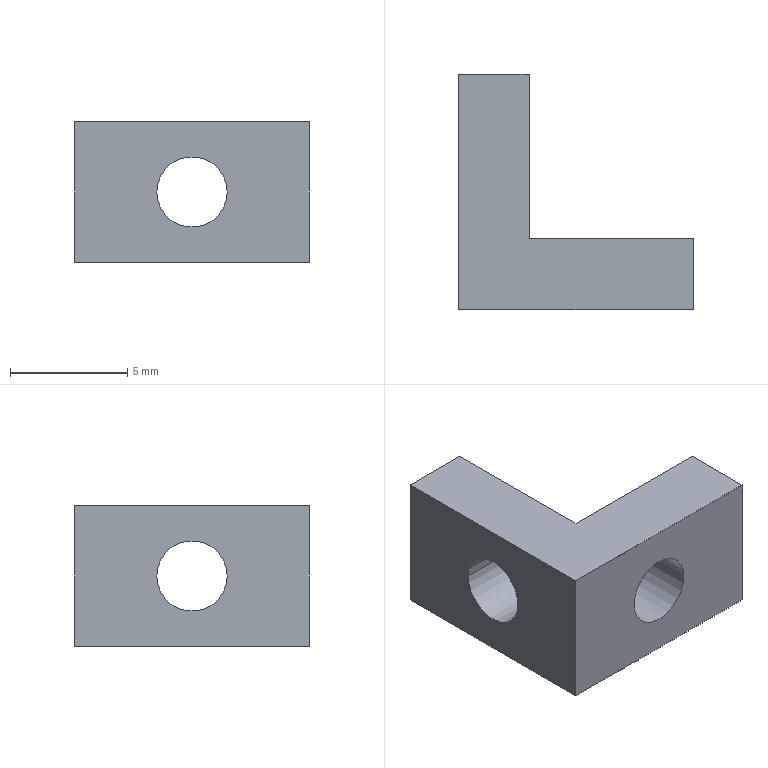Part | SolidWorks | features ICE 2, Extrusion 1 | 1 solid | 12 faces | box 10 x 10 x 6 mm | volume 263.588 mm3 | plane 8 | cylinder 4 | commonest cylinder face diameters 3 x4
STEP:
#1=CARTESIAN_POINT('',(6.5,0.,3.));
#2=VERTEX_POINT('',#1);
#3=CARTESIAN_POINT('',(3.5,0.,3.));
#4=VERTEX_POINT('',#3);
#5=CARTESIAN_POINT('',(5.,0.,3.));
#6=DIRECTION('',(0.,1.,0.));
#7=DIRECTION('',(-1.,0.,0.));
#8=AXIS2_PLACEMENT_3D('',#5,#6,#7);
#9=CIRCLE('',#8,1.5);
#10=EDGE_CURVE('',#2,#4,#9,.T.);
#11=ORIENTED_EDGE('',*,*,#10,.F.);
#12=CARTESIAN_POINT('',(6.5,3.,3.));
#13=VERTEX_POINT('',#12);
#14=CARTESIAN_POINT('',(6.5,0.,3.));
#15=DIRECTION('',(0.,1.,0.));
#16=VECTOR('',#15,1000.);
#17=LINE('',#14,#16);
#18=EDGE_CURVE('',#2,#13,#17,.T.);
#19=ORIENTED_EDGE('',*,*,#18,.T.);
#20=CARTESIAN_POINT('',(3.5,3.,3.));
#21=VERTEX_POINT('',#20);
#22=CARTESIAN_POINT('',(5.,3.,3.));
#23=DIRECTION('',(0.,1.,0.));
#24=DIRECTION('',(-1.,0.,0.));
#25=AXIS2_PLACEMENT_3D('',#22,#23,#24);
#26=CIRCLE('',#25,1.5);
#27=EDGE_CURVE('',#13,#21,#26,.T.);
#28=ORIENTED_EDGE('',*,*,#27,.T.);
#29=CARTESIAN_POINT('',(3.5,0.,3.));
#30=DIRECTION('',(0.,1.,0.));
#31=VECTOR('',#30,1000.);
#32=LINE('',#29,#31);
#33=EDGE_CURVE('',#4,#21,#32,.T.);
#34=ORIENTED_EDGE('',*,*,#33,.F.);
#35=EDGE_LOOP('',(#11,#19,#28,#34));
#36=FACE_OUTER_BOUND('',#35,.T.);
#37=CARTESIAN_POINT('',(5.,0.,3.));
#38=DIRECTION('',(0.,1.,0.));
#39=DIRECTION('',(-1.,0.,0.));
#40=AXIS2_PLACEMENT_3D('',#37,#38,#39);
#41=CYLINDRICAL_SURFACE('',#40,1.5);
#42=ADVANCED_FACE('',(#36),#41,.F.);
#43=CARTESIAN_POINT('',(0.,3.5,3.));
#44=VERTEX_POINT('',#43);
#45=CARTESIAN_POINT('',(0.,6.5,3.));
#46=VERTEX_POINT('',#45);
#47=CARTESIAN_POINT('',(0.,5.,3.));
#48=DIRECTION('',(1.,0.,0.));
#49=DIRECTION('',(0.,1.,0.));
#50=AXIS2_PLACEMENT_3D('',#47,#48,#49);
#51=CIRCLE('',#50,1.5);
#52=EDGE_CURVE('',#44,#46,#51,.T.);
#53=ORIENTED_EDGE('',*,*,#52,.F.);
#54=CARTESIAN_POINT('',(3.,3.5,3.));
#55=VERTEX_POINT('',#54);
#56=CARTESIAN_POINT('',(0.,3.5,3.));
#57=DIRECTION('',(1.,0.,0.));
#58=VECTOR('',#57,1000.);
#59=LINE('',#56,#58);
#60=EDGE_CURVE('',#44,#55,#59,.T.);
#61=ORIENTED_EDGE('',*,*,#60,.T.);
#62=CARTESIAN_POINT('',(3.,6.5,3.));
#63=VERTEX_POINT('',#62);
#64=CARTESIAN_POINT('',(3.,5.,3.));
#65=DIRECTION('',(1.,0.,0.));
#66=DIRECTION('',(0.,1.,0.));
#67=AXIS2_PLACEMENT_3D('',#64,#65,#66);
#68=CIRCLE('',#67,1.5);
#69=EDGE_CURVE('',#55,#63,#68,.T.);
#70=ORIENTED_EDGE('',*,*,#69,.T.);
#71=CARTESIAN_POINT('',(0.,6.5,3.));
#72=DIRECTION('',(1.,0.,0.));
#73=VECTOR('',#72,1000.);
#74=LINE('',#71,#73);
#75=EDGE_CURVE('',#46,#63,#74,.T.);
#76=ORIENTED_EDGE('',*,*,#75,.F.);
#77=EDGE_LOOP('',(#53,#61,#70,#76));
#78=FACE_OUTER_BOUND('',#77,.T.);
#79=CARTESIAN_POINT('',(0.,5.,3.));
#80=DIRECTION('',(1.,0.,0.));
#81=DIRECTION('',(0.,1.,0.));
#82=AXIS2_PLACEMENT_3D('',#79,#80,#81);
#83=CYLINDRICAL_SURFACE('',#82,1.5);
#84=ADVANCED_FACE('',(#78),#83,.F.);
#85=CARTESIAN_POINT('',(0.,5.,3.));
#86=DIRECTION('',(1.,0.,0.));
#87=DIRECTION('',(0.,1.,0.));
#88=AXIS2_PLACEMENT_3D('',#85,#86,#87);
#89=CIRCLE('',#88,1.5);
#90=EDGE_CURVE('',#46,#44,#89,.T.);
#91=ORIENTED_EDGE('',*,*,#90,.T.);
#92=ORIENTED_EDGE('',*,*,#52,.T.);
#93=EDGE_LOOP('',(#91,#92));
#94=FACE_BOUND('',#93,.T.);
#95=CARTESIAN_POINT('',(0.,10.,0.));
#96=VERTEX_POINT('',#95);
#97=CARTESIAN_POINT('',(0.,0.,0.));
#98=VERTEX_POINT('',#97);
#99=CARTESIAN_POINT('',(0.,10.,0.));
#100=DIRECTION('',(0.,-1.,0.));
#101=VECTOR('',#100,1000.);
#102=LINE('',#99,#101);
#103=EDGE_CURVE('',#96,#98,#102,.T.);
#104=ORIENTED_EDGE('',*,*,#103,.T.);
#105=CARTESIAN_POINT('',(0.,0.,6.));
#106=VERTEX_POINT('',#105);
#107=CARTESIAN_POINT('',(0.,0.,6.));
#108=DIRECTION('',(0.,0.,-1.));
#109=VECTOR('',#108,1000.);
#110=LINE('',#107,#109);
#111=EDGE_CURVE('',#106,#98,#110,.T.);
#112=ORIENTED_EDGE('',*,*,#111,.F.);
#113=CARTESIAN_POINT('',(0.,10.,6.));
#114=VERTEX_POINT('',#113);
#115=CARTESIAN_POINT('',(0.,10.,6.));
#116=DIRECTION('',(0.,-1.,0.));
#117=VECTOR('',#116,1000.);
#118=LINE('',#115,#117);
#119=EDGE_CURVE('',#114,#106,#118,.T.);
#120=ORIENTED_EDGE('',*,*,#119,.F.);
#121=CARTESIAN_POINT('',(0.,10.,6.));
#122=DIRECTION('',(0.,0.,-1.));
#123=VECTOR('',#122,1000.);
#124=LINE('',#121,#123);
#125=EDGE_CURVE('',#114,#96,#124,.T.);
#126=ORIENTED_EDGE('',*,*,#125,.T.);
#127=EDGE_LOOP('',(#104,#112,#120,#126));
#128=FACE_OUTER_BOUND('',#127,.T.);
#129=CARTESIAN_POINT('',(0.,10.,6.));
#130=DIRECTION('',(1.,0.,0.));
#131=DIRECTION('',(0.,1.,0.));
#132=AXIS2_PLACEMENT_3D('',#129,#130,#131);
#133=PLANE('',#132);
#134=ADVANCED_FACE('',(#94,#128),#133,.F.);
#135=CARTESIAN_POINT('',(5.,0.,3.));
#136=DIRECTION('',(0.,1.,0.));
#137=DIRECTION('',(-1.,0.,0.));
#138=AXIS2_PLACEMENT_3D('',#135,#136,#137);
#139=CIRCLE('',#138,1.5);
#140=EDGE_CURVE('',#4,#2,#139,.T.);
#141=ORIENTED_EDGE('',*,*,#140,.T.);
#142=ORIENTED_EDGE('',*,*,#10,.T.);
#143=EDGE_LOOP('',(#141,#142));
#144=FACE_BOUND('',#143,.T.);
#145=CARTESIAN_POINT('',(10.,0.,0.));
#146=VERTEX_POINT('',#145);
#147=CARTESIAN_POINT('',(0.,0.,0.));
#148=DIRECTION('',(1.,0.,0.));
#149=VECTOR('',#148,1000.);
#150=LINE('',#147,#149);
#151=EDGE_CURVE('',#98,#146,#150,.T.);
#152=ORIENTED_EDGE('',*,*,#151,.T.);
#153=CARTESIAN_POINT('',(10.,0.,6.));
#154=VERTEX_POINT('',#153);
#155=CARTESIAN_POINT('',(10.,0.,6.));
#156=DIRECTION('',(0.,0.,-1.));
#157=VECTOR('',#156,1000.);
#158=LINE('',#155,#157);
#159=EDGE_CURVE('',#154,#146,#158,.T.);
#160=ORIENTED_EDGE('',*,*,#159,.F.);
#161=CARTESIAN_POINT('',(0.,0.,6.));
#162=DIRECTION('',(1.,0.,0.));
#163=VECTOR('',#162,1000.);
#164=LINE('',#161,#163);
#165=EDGE_CURVE('',#106,#154,#164,.T.);
#166=ORIENTED_EDGE('',*,*,#165,.F.);
#167=ORIENTED_EDGE('',*,*,#111,.T.);
#168=EDGE_LOOP('',(#152,#160,#166,#167));
#169=FACE_OUTER_BOUND('',#168,.T.);
#170=CARTESIAN_POINT('',(0.,0.,6.));
#171=DIRECTION('',(0.,1.,0.));
#172=DIRECTION('',(0.,0.,1.));
#173=AXIS2_PLACEMENT_3D('',#170,#171,#172);
#174=PLANE('',#173);
#175=ADVANCED_FACE('',(#144,#169),#174,.F.);
#176=CARTESIAN_POINT('',(10.,3.,0.));
#177=VERTEX_POINT('',#176);
#178=CARTESIAN_POINT('',(10.,0.,0.));
#179=DIRECTION('',(0.,1.,0.));
#180=VECTOR('',#179,1000.);
#181=LINE('',#178,#180);
#182=EDGE_CURVE('',#146,#177,#181,.T.);
#183=ORIENTED_EDGE('',*,*,#182,.T.);
#184=CARTESIAN_POINT('',(10.,3.,6.));
#185=VERTEX_POINT('',#184);
#186=CARTESIAN_POINT('',(10.,3.,6.));
#187=DIRECTION('',(0.,0.,-1.));
#188=VECTOR('',#187,1000.);
#189=LINE('',#186,#188);
#190=EDGE_CURVE('',#185,#177,#189,.T.);
#191=ORIENTED_EDGE('',*,*,#190,.F.);
#192=CARTESIAN_POINT('',(10.,0.,6.));
#193=DIRECTION('',(0.,1.,0.));
#194=VECTOR('',#193,1000.);
#195=LINE('',#192,#194);
#196=EDGE_CURVE('',#154,#185,#195,.T.);
#197=ORIENTED_EDGE('',*,*,#196,.F.);
#198=ORIENTED_EDGE('',*,*,#159,.T.);
#199=EDGE_LOOP('',(#183,#191,#197,#198));
#200=FACE_OUTER_BOUND('',#199,.T.);
#201=CARTESIAN_POINT('',(10.,0.,6.));
#202=DIRECTION('',(-1.,0.,0.));
#203=DIRECTION('',(0.,0.,1.));
#204=AXIS2_PLACEMENT_3D('',#201,#202,#203);
#205=PLANE('',#204);
#206=ADVANCED_FACE('',(#200),#205,.F.);
#207=CARTESIAN_POINT('',(5.,3.,3.));
#208=DIRECTION('',(0.,1.,0.));
#209=DIRECTION('',(-1.,0.,0.));
#210=AXIS2_PLACEMENT_3D('',#207,#208,#209);
#211=CIRCLE('',#210,1.5);
#212=EDGE_CURVE('',#21,#13,#211,.T.);
#213=ORIENTED_EDGE('',*,*,#212,.F.);
#214=ORIENTED_EDGE('',*,*,#27,.F.);
#215=EDGE_LOOP('',(#213,#214));
#216=FACE_BOUND('',#215,.T.);
#217=CARTESIAN_POINT('',(3.,3.,0.));
#218=VERTEX_POINT('',#217);
#219=CARTESIAN_POINT('',(10.,3.,0.));
#220=DIRECTION('',(-1.,0.,0.));
#221=VECTOR('',#220,1000.);
#222=LINE('',#219,#221);
#223=EDGE_CURVE('',#177,#218,#222,.T.);
#224=ORIENTED_EDGE('',*,*,#223,.T.);
#225=CARTESIAN_POINT('',(3.,3.,6.));
#226=VERTEX_POINT('',#225);
#227=CARTESIAN_POINT('',(3.,3.,6.));
#228=DIRECTION('',(0.,0.,-1.));
#229=VECTOR('',#228,1000.);
#230=LINE('',#227,#229);
#231=EDGE_CURVE('',#226,#218,#230,.T.);
#232=ORIENTED_EDGE('',*,*,#231,.F.);
#233=CARTESIAN_POINT('',(10.,3.,6.));
#234=DIRECTION('',(-1.,0.,0.));
#235=VECTOR('',#234,1000.);
#236=LINE('',#233,#235);
#237=EDGE_CURVE('',#185,#226,#236,.T.);
#238=ORIENTED_EDGE('',*,*,#237,.F.);
#239=ORIENTED_EDGE('',*,*,#190,.T.);
#240=EDGE_LOOP('',(#224,#232,#238,#239));
#241=FACE_OUTER_BOUND('',#240,.T.);
#242=CARTESIAN_POINT('',(10.,3.,6.));
#243=DIRECTION('',(0.,-1.,0.));
#244=DIRECTION('',(1.,0.,0.));
#245=AXIS2_PLACEMENT_3D('',#242,#243,#244);
#246=PLANE('',#245);
#247=ADVANCED_FACE('',(#216,#241),#246,.F.);
#248=CARTESIAN_POINT('',(3.,5.,3.));
#249=DIRECTION('',(1.,0.,0.));
#250=DIRECTION('',(0.,1.,0.));
#251=AXIS2_PLACEMENT_3D('',#248,#249,#250);
#252=CIRCLE('',#251,1.5);
#253=EDGE_CURVE('',#63,#55,#252,.T.);
#254=ORIENTED_EDGE('',*,*,#253,.F.);
#255=ORIENTED_EDGE('',*,*,#69,.F.);
#256=EDGE_LOOP('',(#254,#255));
#257=FACE_BOUND('',#256,.T.);
#258=CARTESIAN_POINT('',(3.,10.,0.));
#259=VERTEX_POINT('',#258);
#260=CARTESIAN_POINT('',(3.,3.,0.));
#261=DIRECTION('',(0.,1.,0.));
#262=VECTOR('',#261,1000.);
#263=LINE('',#260,#262);
#264=EDGE_CURVE('',#218,#259,#263,.T.);
#265=ORIENTED_EDGE('',*,*,#264,.T.);
#266=CARTESIAN_POINT('',(3.,10.,6.));
#267=VERTEX_POINT('',#266);
#268=CARTESIAN_POINT('',(3.,10.,6.));
#269=DIRECTION('',(0.,0.,-1.));
#270=VECTOR('',#269,1000.);
#271=LINE('',#268,#270);
#272=EDGE_CURVE('',#267,#259,#271,.T.);
#273=ORIENTED_EDGE('',*,*,#272,.F.);
#274=CARTESIAN_POINT('',(3.,3.,6.));
#275=DIRECTION('',(0.,1.,0.));
#276=VECTOR('',#275,1000.);
#277=LINE('',#274,#276);
#278=EDGE_CURVE('',#226,#267,#277,.T.);
#279=ORIENTED_EDGE('',*,*,#278,.F.);
#280=ORIENTED_EDGE('',*,*,#231,.T.);
#281=EDGE_LOOP('',(#265,#273,#279,#280));
#282=FACE_OUTER_BOUND('',#281,.T.);
#283=CARTESIAN_POINT('',(3.,3.,6.));
#284=DIRECTION('',(-1.,0.,0.));
#285=DIRECTION('',(0.,-1.,0.));
#286=AXIS2_PLACEMENT_3D('',#283,#284,#285);
#287=PLANE('',#286);
#288=ADVANCED_FACE('',(#257,#282),#287,.F.);
#289=CARTESIAN_POINT('',(3.,10.,0.));
#290=DIRECTION('',(-1.,0.,0.));
#291=VECTOR('',#290,1000.);
#292=LINE('',#289,#291);
#293=EDGE_CURVE('',#259,#96,#292,.T.);
#294=ORIENTED_EDGE('',*,*,#293,.T.);
#295=ORIENTED_EDGE('',*,*,#125,.F.);
#296=CARTESIAN_POINT('',(3.,10.,6.));
#297=DIRECTION('',(-1.,0.,0.));
#298=VECTOR('',#297,1000.);
#299=LINE('',#296,#298);
#300=EDGE_CURVE('',#267,#114,#299,.T.);
#301=ORIENTED_EDGE('',*,*,#300,.F.);
#302=ORIENTED_EDGE('',*,*,#272,.T.);
#303=EDGE_LOOP('',(#294,#295,#301,#302));
#304=FACE_OUTER_BOUND('',#303,.T.);
#305=CARTESIAN_POINT('',(3.,10.,6.));
#306=DIRECTION('',(0.,-1.,0.));
#307=DIRECTION('',(0.,0.,-1.));
#308=AXIS2_PLACEMENT_3D('',#305,#306,#307);
#309=PLANE('',#308);
#310=ADVANCED_FACE('',(#304),#309,.F.);
#311=ORIENTED_EDGE('',*,*,#119,.T.);
#312=ORIENTED_EDGE('',*,*,#165,.T.);
#313=ORIENTED_EDGE('',*,*,#196,.T.);
#314=ORIENTED_EDGE('',*,*,#237,.T.);
#315=ORIENTED_EDGE('',*,*,#278,.T.);
#316=ORIENTED_EDGE('',*,*,#300,.T.);
#317=EDGE_LOOP('',(#311,#312,#313,#314,#315,#316));
#318=FACE_OUTER_BOUND('',#317,.T.);
#319=CARTESIAN_POINT('',(0.,0.,6.));
#320=DIRECTION('',(0.,0.,1.));
#321=DIRECTION('',(1.,0.,0.));
#322=AXIS2_PLACEMENT_3D('',#319,#320,#321);
#323=PLANE('',#322);
#324=ADVANCED_FACE('',(#318),#323,.T.);
#325=ORIENTED_EDGE('',*,*,#103,.F.);
#326=ORIENTED_EDGE('',*,*,#293,.F.);
#327=ORIENTED_EDGE('',*,*,#264,.F.);
#328=ORIENTED_EDGE('',*,*,#223,.F.);
#329=ORIENTED_EDGE('',*,*,#182,.F.);
#330=ORIENTED_EDGE('',*,*,#151,.F.);
#331=EDGE_LOOP('',(#325,#326,#327,#328,#329,#330));
#332=FACE_OUTER_BOUND('',#331,.T.);
#333=CARTESIAN_POINT('',(0.,0.,0.));
#334=DIRECTION('',(0.,0.,1.));
#335=DIRECTION('',(1.,0.,0.));
#336=AXIS2_PLACEMENT_3D('',#333,#334,#335);
#337=PLANE('',#336);
#338=ADVANCED_FACE('',(#332),#337,.F.);
#339=ORIENTED_EDGE('',*,*,#60,.F.);
#340=ORIENTED_EDGE('',*,*,#90,.F.);
#341=ORIENTED_EDGE('',*,*,#75,.T.);
#342=ORIENTED_EDGE('',*,*,#253,.T.);
#343=EDGE_LOOP('',(#339,#340,#341,#342));
#344=FACE_OUTER_BOUND('',#343,.T.);
#345=CARTESIAN_POINT('',(0.,5.,3.));
#346=DIRECTION('',(1.,0.,0.));
#347=DIRECTION('',(0.,1.,0.));
#348=AXIS2_PLACEMENT_3D('',#345,#346,#347);
#349=CYLINDRICAL_SURFACE('',#348,1.5);
#350=ADVANCED_FACE('',(#344),#349,.F.);
#351=ORIENTED_EDGE('',*,*,#18,.F.);
#352=ORIENTED_EDGE('',*,*,#140,.F.);
#353=ORIENTED_EDGE('',*,*,#33,.T.);
#354=ORIENTED_EDGE('',*,*,#212,.T.);
#355=EDGE_LOOP('',(#351,#352,#353,#354));
#356=FACE_OUTER_BOUND('',#355,.T.);
#357=CARTESIAN_POINT('',(5.,0.,3.));
#358=DIRECTION('',(0.,1.,0.));
#359=DIRECTION('',(-1.,0.,0.));
#360=AXIS2_PLACEMENT_3D('',#357,#358,#359);
#361=CYLINDRICAL_SURFACE('',#360,1.5);
#362=ADVANCED_FACE('',(#356),#361,.F.);
#363=CLOSED_SHELL('',(#42,#84,#134,#175,#206,#247,#288,#310,#324,#338,#350,#362));
#364=MANIFOLD_SOLID_BREP('',#363);
#365=CARTESIAN_POINT('',(0.,0.,0.));
#366=DIRECTION('',(0.,0.,1.));
#367=DIRECTION('',(1.,0.,0.));
#368=AXIS2_PLACEMENT_3D('',#365,#366,#367);
#369=(LENGTH_UNIT()NAMED_UNIT(*)SI_UNIT(.MILLI.,.METRE.));
#370=UNCERTAINTY_MEASURE_WITH_UNIT(LENGTH_MEASURE(0.00001),#369,'','');
#371=(NAMED_UNIT(*)PLANE_ANGLE_UNIT()SI_UNIT($,.RADIAN.));
#372=(NAMED_UNIT(*)SI_UNIT($,.STERADIAN.)SOLID_ANGLE_UNIT());
#373=(GEOMETRIC_REPRESENTATION_CONTEXT(3)GLOBAL_UNCERTAINTY_ASSIGNED_CONTEXT((#370))GLOBAL_UNIT_ASSIGNED_CONTEXT((#369,#371,#372))REPRESENTATION_CONTEXT('',''));
#374=ADVANCED_BREP_SHAPE_REPRESENTATION('',(#364,#368),#373);